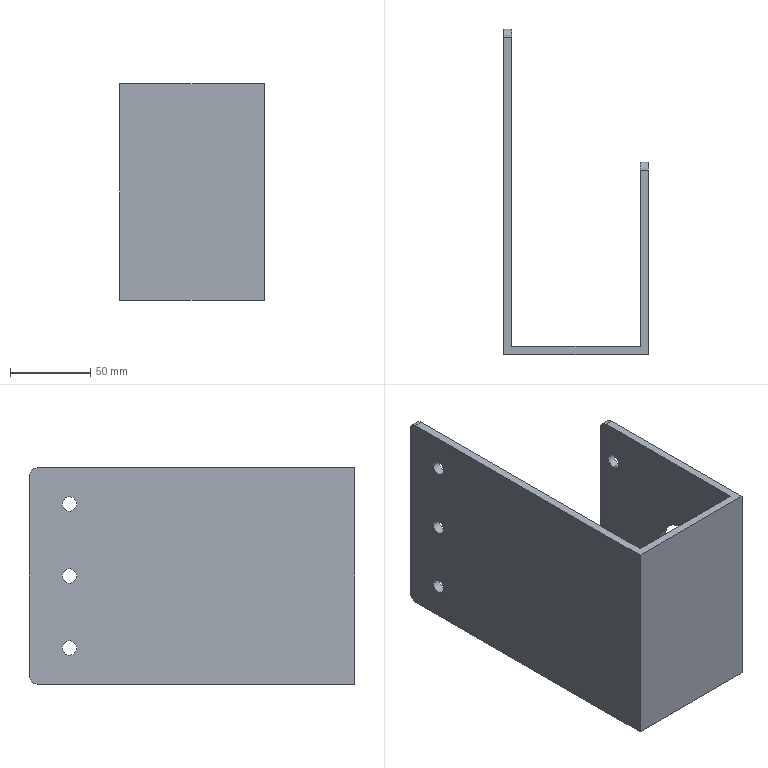Part | SolidWorks | features ICE 2, ExtruThin 1, Fillet 1 | 1 solid | 30 faces | box 90 x 203 x 135 mm | volume 261739 mm3 | cylinder 20 | plane 10 | commonest cylinder face diameters 9 x14 10 x4 45 x2
STEP:
#1=CARTESIAN_POINT('',(-35.,-32.5,-45.));
#2=VERTEX_POINT('',#1);
#3=CARTESIAN_POINT('',(-35.,-41.5,-45.));
#4=VERTEX_POINT('',#3);
#5=CARTESIAN_POINT('',(-35.,-37.,-45.));
#6=DIRECTION('',(-1.,0.,0.));
#7=DIRECTION('',(0.,1.,0.));
#8=AXIS2_PLACEMENT_3D('',#5,#6,#7);
#9=CIRCLE('',#8,4.5);
#10=EDGE_CURVE('',#2,#4,#9,.T.);
#11=ORIENTED_EDGE('',*,*,#10,.F.);
#12=CARTESIAN_POINT('',(-40.,-32.5,-45.));
#13=VERTEX_POINT('',#12);
#14=CARTESIAN_POINT('',(-30.,-32.5,-45.));
#15=DIRECTION('',(-1.,0.,0.));
#16=VECTOR('',#15,1000.);
#17=LINE('',#14,#16);
#18=EDGE_CURVE('',#2,#13,#17,.T.);
#19=ORIENTED_EDGE('',*,*,#18,.T.);
#20=CARTESIAN_POINT('',(-40.,-41.5,-45.));
#21=VERTEX_POINT('',#20);
#22=CARTESIAN_POINT('',(-40.,-37.,-45.));
#23=DIRECTION('',(1.,0.,0.));
#24=DIRECTION('',(0.,1.,0.));
#25=AXIS2_PLACEMENT_3D('',#22,#23,#24);
#26=CIRCLE('',#25,4.5);
#27=EDGE_CURVE('',#21,#13,#26,.T.);
#28=ORIENTED_EDGE('',*,*,#27,.F.);
#29=CARTESIAN_POINT('',(-30.,-41.5,-45.));
#30=DIRECTION('',(-1.,0.,0.));
#31=VECTOR('',#30,1000.);
#32=LINE('',#29,#31);
#33=EDGE_CURVE('',#4,#21,#32,.T.);
#34=ORIENTED_EDGE('',*,*,#33,.F.);
#35=EDGE_LOOP('',(#11,#19,#28,#34));
#36=FACE_OUTER_BOUND('',#35,.T.);
#37=CARTESIAN_POINT('',(-30.,-37.,-45.));
#38=DIRECTION('',(-1.,0.,0.));
#39=DIRECTION('',(0.,-1.,0.));
#40=AXIS2_PLACEMENT_3D('',#37,#38,#39);
#41=CYLINDRICAL_SURFACE('',#40,4.5);
#42=ADVANCED_FACE('',(#36),#41,.F.);
#43=CARTESIAN_POINT('',(-35.,-32.5,45.));
#44=VERTEX_POINT('',#43);
#45=CARTESIAN_POINT('',(-35.,-41.5,45.));
#46=VERTEX_POINT('',#45);
#47=CARTESIAN_POINT('',(-35.,-37.,45.));
#48=DIRECTION('',(-1.,0.,0.));
#49=DIRECTION('',(0.,1.,0.));
#50=AXIS2_PLACEMENT_3D('',#47,#48,#49);
#51=CIRCLE('',#50,4.5);
#52=EDGE_CURVE('',#44,#46,#51,.T.);
#53=ORIENTED_EDGE('',*,*,#52,.F.);
#54=CARTESIAN_POINT('',(-40.,-32.5,45.));
#55=VERTEX_POINT('',#54);
#56=CARTESIAN_POINT('',(-30.,-32.5,45.));
#57=DIRECTION('',(-1.,0.,0.));
#58=VECTOR('',#57,1000.);
#59=LINE('',#56,#58);
#60=EDGE_CURVE('',#44,#55,#59,.T.);
#61=ORIENTED_EDGE('',*,*,#60,.T.);
#62=CARTESIAN_POINT('',(-40.,-41.5,45.));
#63=VERTEX_POINT('',#62);
#64=CARTESIAN_POINT('',(-40.,-37.,45.));
#65=DIRECTION('',(1.,0.,0.));
#66=DIRECTION('',(0.,1.,0.));
#67=AXIS2_PLACEMENT_3D('',#64,#65,#66);
#68=CIRCLE('',#67,4.5);
#69=EDGE_CURVE('',#63,#55,#68,.T.);
#70=ORIENTED_EDGE('',*,*,#69,.F.);
#71=CARTESIAN_POINT('',(-30.,-41.5,45.));
#72=DIRECTION('',(-1.,0.,0.));
#73=VECTOR('',#72,1000.);
#74=LINE('',#71,#73);
#75=EDGE_CURVE('',#46,#63,#74,.T.);
#76=ORIENTED_EDGE('',*,*,#75,.F.);
#77=EDGE_LOOP('',(#53,#61,#70,#76));
#78=FACE_OUTER_BOUND('',#77,.T.);
#79=CARTESIAN_POINT('',(-30.,-37.,45.));
#80=DIRECTION('',(-1.,0.,0.));
#81=DIRECTION('',(0.,-1.,0.));
#82=AXIS2_PLACEMENT_3D('',#79,#80,#81);
#83=CYLINDRICAL_SURFACE('',#82,4.5);
#84=ADVANCED_FACE('',(#78),#83,.F.);
#85=CARTESIAN_POINT('',(-35.,-32.5,0.));
#86=VERTEX_POINT('',#85);
#87=CARTESIAN_POINT('',(-35.,-41.5,0.));
#88=VERTEX_POINT('',#87);
#89=CARTESIAN_POINT('',(-35.,-37.,0.));
#90=DIRECTION('',(-1.,0.,0.));
#91=DIRECTION('',(0.,1.,0.));
#92=AXIS2_PLACEMENT_3D('',#89,#90,#91);
#93=CIRCLE('',#92,4.5);
#94=EDGE_CURVE('',#86,#88,#93,.T.);
#95=ORIENTED_EDGE('',*,*,#94,.F.);
#96=CARTESIAN_POINT('',(-40.,-32.5,0.));
#97=VERTEX_POINT('',#96);
#98=CARTESIAN_POINT('',(-30.,-32.5,0.));
#99=DIRECTION('',(-1.,0.,0.));
#100=VECTOR('',#99,1000.);
#101=LINE('',#98,#100);
#102=EDGE_CURVE('',#86,#97,#101,.T.);
#103=ORIENTED_EDGE('',*,*,#102,.T.);
#104=CARTESIAN_POINT('',(-40.,-41.5,0.));
#105=VERTEX_POINT('',#104);
#106=CARTESIAN_POINT('',(-40.,-37.,0.));
#107=DIRECTION('',(1.,0.,0.));
#108=DIRECTION('',(0.,1.,0.));
#109=AXIS2_PLACEMENT_3D('',#106,#107,#108);
#110=CIRCLE('',#109,4.5);
#111=EDGE_CURVE('',#105,#97,#110,.T.);
#112=ORIENTED_EDGE('',*,*,#111,.F.);
#113=CARTESIAN_POINT('',(-30.,-41.5,0.));
#114=DIRECTION('',(-1.,0.,0.));
#115=VECTOR('',#114,1000.);
#116=LINE('',#113,#115);
#117=EDGE_CURVE('',#88,#105,#116,.T.);
#118=ORIENTED_EDGE('',*,*,#117,.F.);
#119=EDGE_LOOP('',(#95,#103,#112,#118));
#120=FACE_OUTER_BOUND('',#119,.T.);
#121=CARTESIAN_POINT('',(-30.,-37.,0.));
#122=DIRECTION('',(-1.,0.,0.));
#123=DIRECTION('',(0.,-1.,0.));
#124=AXIS2_PLACEMENT_3D('',#121,#122,#123);
#125=CYLINDRICAL_SURFACE('',#124,4.5);
#126=ADVANCED_FACE('',(#120),#125,.F.);
#127=CARTESIAN_POINT('',(45.,-106.574,37.926));
#128=VERTEX_POINT('',#127);
#129=CARTESIAN_POINT('',(45.,-106.574,46.926));
#130=VERTEX_POINT('',#129);
#131=CARTESIAN_POINT('',(45.,-106.574,42.426));
#132=DIRECTION('',(-1.,0.,0.));
#133=DIRECTION('',(0.,0.,1.));
#134=AXIS2_PLACEMENT_3D('',#131,#132,#133);
#135=CIRCLE('',#134,4.5);
#136=EDGE_CURVE('',#128,#130,#135,.T.);
#137=ORIENTED_EDGE('',*,*,#136,.T.);
#138=CARTESIAN_POINT('',(50.,-106.574,46.926));
#139=VERTEX_POINT('',#138);
#140=CARTESIAN_POINT('',(40.,-106.574,46.926));
#141=DIRECTION('',(1.,0.,0.));
#142=VECTOR('',#141,1000.);
#143=LINE('',#140,#142);
#144=EDGE_CURVE('',#130,#139,#143,.T.);
#145=ORIENTED_EDGE('',*,*,#144,.T.);
#146=CARTESIAN_POINT('',(50.,-106.574,37.926));
#147=VERTEX_POINT('',#146);
#148=CARTESIAN_POINT('',(50.,-106.574,42.426));
#149=DIRECTION('',(1.,0.,0.));
#150=DIRECTION('',(0.,0.,-1.));
#151=AXIS2_PLACEMENT_3D('',#148,#149,#150);
#152=CIRCLE('',#151,4.5);
#153=EDGE_CURVE('',#139,#147,#152,.T.);
#154=ORIENTED_EDGE('',*,*,#153,.T.);
#155=CARTESIAN_POINT('',(40.,-106.574,37.926));
#156=DIRECTION('',(1.,0.,0.));
#157=VECTOR('',#156,1000.);
#158=LINE('',#155,#157);
#159=EDGE_CURVE('',#128,#147,#158,.T.);
#160=ORIENTED_EDGE('',*,*,#159,.F.);
#161=EDGE_LOOP('',(#137,#145,#154,#160));
#162=FACE_OUTER_BOUND('',#161,.T.);
#163=CARTESIAN_POINT('',(40.,-106.574,42.426));
#164=DIRECTION('',(1.,0.,0.));
#165=DIRECTION('',(0.,0.,-1.));
#166=AXIS2_PLACEMENT_3D('',#163,#164,#165);
#167=CYLINDRICAL_SURFACE('',#166,4.5);
#168=ADVANCED_FACE('',(#162),#167,.F.);
#169=CARTESIAN_POINT('',(45.,-191.426,37.926));
#170=VERTEX_POINT('',#169);
#171=CARTESIAN_POINT('',(45.,-191.426,46.926));
#172=VERTEX_POINT('',#171);
#173=CARTESIAN_POINT('',(45.,-191.426,42.426));
#174=DIRECTION('',(-1.,0.,0.));
#175=DIRECTION('',(0.,0.,1.));
#176=AXIS2_PLACEMENT_3D('',#173,#174,#175);
#177=CIRCLE('',#176,4.5);
#178=EDGE_CURVE('',#170,#172,#177,.T.);
#179=ORIENTED_EDGE('',*,*,#178,.T.);
#180=CARTESIAN_POINT('',(50.,-191.426,46.926));
#181=VERTEX_POINT('',#180);
#182=CARTESIAN_POINT('',(40.,-191.426,46.926));
#183=DIRECTION('',(1.,0.,0.));
#184=VECTOR('',#183,1000.);
#185=LINE('',#182,#184);
#186=EDGE_CURVE('',#172,#181,#185,.T.);
#187=ORIENTED_EDGE('',*,*,#186,.T.);
#188=CARTESIAN_POINT('',(50.,-191.426,37.926));
#189=VERTEX_POINT('',#188);
#190=CARTESIAN_POINT('',(50.,-191.426,42.426));
#191=DIRECTION('',(1.,0.,0.));
#192=DIRECTION('',(0.,0.,-1.));
#193=AXIS2_PLACEMENT_3D('',#190,#191,#192);
#194=CIRCLE('',#193,4.5);
#195=EDGE_CURVE('',#181,#189,#194,.T.);
#196=ORIENTED_EDGE('',*,*,#195,.T.);
#197=CARTESIAN_POINT('',(40.,-191.426,37.926));
#198=DIRECTION('',(1.,0.,0.));
#199=VECTOR('',#198,1000.);
#200=LINE('',#197,#199);
#201=EDGE_CURVE('',#170,#189,#200,.T.);
#202=ORIENTED_EDGE('',*,*,#201,.F.);
#203=EDGE_LOOP('',(#179,#187,#196,#202));
#204=FACE_OUTER_BOUND('',#203,.T.);
#205=CARTESIAN_POINT('',(40.,-191.426,42.426));
#206=DIRECTION('',(1.,0.,0.));
#207=DIRECTION('',(0.,0.,-1.));
#208=AXIS2_PLACEMENT_3D('',#205,#206,#207);
#209=CYLINDRICAL_SURFACE('',#208,4.5);
#210=ADVANCED_FACE('',(#204),#209,.F.);
#211=CARTESIAN_POINT('',(45.,-191.426,-46.926));
#212=VERTEX_POINT('',#211);
#213=CARTESIAN_POINT('',(45.,-191.426,-37.926));
#214=VERTEX_POINT('',#213);
#215=CARTESIAN_POINT('',(45.,-191.426,-42.426));
#216=DIRECTION('',(-1.,0.,0.));
#217=DIRECTION('',(0.,0.,1.));
#218=AXIS2_PLACEMENT_3D('',#215,#216,#217);
#219=CIRCLE('',#218,4.5);
#220=EDGE_CURVE('',#212,#214,#219,.T.);
#221=ORIENTED_EDGE('',*,*,#220,.T.);
#222=CARTESIAN_POINT('',(50.,-191.426,-37.926));
#223=VERTEX_POINT('',#222);
#224=CARTESIAN_POINT('',(40.,-191.426,-37.926));
#225=DIRECTION('',(1.,0.,0.));
#226=VECTOR('',#225,1000.);
#227=LINE('',#224,#226);
#228=EDGE_CURVE('',#214,#223,#227,.T.);
#229=ORIENTED_EDGE('',*,*,#228,.T.);
#230=CARTESIAN_POINT('',(50.,-191.426,-46.926));
#231=VERTEX_POINT('',#230);
#232=CARTESIAN_POINT('',(50.,-191.426,-42.426));
#233=DIRECTION('',(1.,0.,0.));
#234=DIRECTION('',(0.,0.,-1.));
#235=AXIS2_PLACEMENT_3D('',#232,#233,#234);
#236=CIRCLE('',#235,4.5);
#237=EDGE_CURVE('',#223,#231,#236,.T.);
#238=ORIENTED_EDGE('',*,*,#237,.T.);
#239=CARTESIAN_POINT('',(40.,-191.426,-46.926));
#240=DIRECTION('',(1.,0.,0.));
#241=VECTOR('',#240,1000.);
#242=LINE('',#239,#241);
#243=EDGE_CURVE('',#212,#231,#242,.T.);
#244=ORIENTED_EDGE('',*,*,#243,.F.);
#245=EDGE_LOOP('',(#221,#229,#238,#244));
#246=FACE_OUTER_BOUND('',#245,.T.);
#247=CARTESIAN_POINT('',(40.,-191.426,-42.426));
#248=DIRECTION('',(1.,0.,0.));
#249=DIRECTION('',(0.,0.,-1.));
#250=AXIS2_PLACEMENT_3D('',#247,#248,#249);
#251=CYLINDRICAL_SURFACE('',#250,4.5);
#252=ADVANCED_FACE('',(#246),#251,.F.);
#253=CARTESIAN_POINT('',(45.,-106.574,-46.926));
#254=VERTEX_POINT('',#253);
#255=CARTESIAN_POINT('',(45.,-106.574,-37.926));
#256=VERTEX_POINT('',#255);
#257=CARTESIAN_POINT('',(45.,-106.574,-42.426));
#258=DIRECTION('',(-1.,0.,0.));
#259=DIRECTION('',(0.,0.,1.));
#260=AXIS2_PLACEMENT_3D('',#257,#258,#259);
#261=CIRCLE('',#260,4.5);
#262=EDGE_CURVE('',#254,#256,#261,.T.);
#263=ORIENTED_EDGE('',*,*,#262,.T.);
#264=CARTESIAN_POINT('',(50.,-106.574,-37.926));
#265=VERTEX_POINT('',#264);
#266=CARTESIAN_POINT('',(40.,-106.574,-37.926));
#267=DIRECTION('',(1.,0.,0.));
#268=VECTOR('',#267,1000.);
#269=LINE('',#266,#268);
#270=EDGE_CURVE('',#256,#265,#269,.T.);
#271=ORIENTED_EDGE('',*,*,#270,.T.);
#272=CARTESIAN_POINT('',(50.,-106.574,-46.926));
#273=VERTEX_POINT('',#272);
#274=CARTESIAN_POINT('',(50.,-106.574,-42.426));
#275=DIRECTION('',(1.,0.,0.));
#276=DIRECTION('',(0.,0.,-1.));
#277=AXIS2_PLACEMENT_3D('',#274,#275,#276);
#278=CIRCLE('',#277,4.5);
#279=EDGE_CURVE('',#265,#273,#278,.T.);
#280=ORIENTED_EDGE('',*,*,#279,.T.);
#281=CARTESIAN_POINT('',(40.,-106.574,-46.926));
#282=DIRECTION('',(1.,0.,0.));
#283=VECTOR('',#282,1000.);
#284=LINE('',#281,#283);
#285=EDGE_CURVE('',#254,#273,#284,.T.);
#286=ORIENTED_EDGE('',*,*,#285,.F.);
#287=EDGE_LOOP('',(#263,#271,#280,#286));
#288=FACE_OUTER_BOUND('',#287,.T.);
#289=CARTESIAN_POINT('',(40.,-106.574,-42.426));
#290=DIRECTION('',(1.,0.,0.));
#291=DIRECTION('',(0.,0.,-1.));
#292=AXIS2_PLACEMENT_3D('',#289,#290,#291);
#293=CYLINDRICAL_SURFACE('',#292,4.5);
#294=ADVANCED_FACE('',(#288),#293,.F.);
#295=CARTESIAN_POINT('',(45.,-169.,-22.5));
#296=VERTEX_POINT('',#295);
#297=CARTESIAN_POINT('',(45.,-169.,22.5));
#298=VERTEX_POINT('',#297);
#299=CARTESIAN_POINT('',(45.,-169.,0.));
#300=DIRECTION('',(-1.,0.,0.));
#301=DIRECTION('',(0.,0.,1.));
#302=AXIS2_PLACEMENT_3D('',#299,#300,#301);
#303=CIRCLE('',#302,22.5);
#304=EDGE_CURVE('',#296,#298,#303,.T.);
#305=ORIENTED_EDGE('',*,*,#304,.T.);
#306=CARTESIAN_POINT('',(50.,-169.,22.5));
#307=VERTEX_POINT('',#306);
#308=CARTESIAN_POINT('',(40.,-169.,22.5));
#309=DIRECTION('',(1.,0.,0.));
#310=VECTOR('',#309,1000.);
#311=LINE('',#308,#310);
#312=EDGE_CURVE('',#298,#307,#311,.T.);
#313=ORIENTED_EDGE('',*,*,#312,.T.);
#314=CARTESIAN_POINT('',(50.,-169.,-22.5));
#315=VERTEX_POINT('',#314);
#316=CARTESIAN_POINT('',(50.,-169.,0.));
#317=DIRECTION('',(1.,0.,0.));
#318=DIRECTION('',(0.,0.,-1.));
#319=AXIS2_PLACEMENT_3D('',#316,#317,#318);
#320=CIRCLE('',#319,22.5);
#321=EDGE_CURVE('',#307,#315,#320,.T.);
#322=ORIENTED_EDGE('',*,*,#321,.T.);
#323=CARTESIAN_POINT('',(40.,-169.,-22.5));
#324=DIRECTION('',(1.,0.,0.));
#325=VECTOR('',#324,1000.);
#326=LINE('',#323,#325);
#327=EDGE_CURVE('',#296,#315,#326,.T.);
#328=ORIENTED_EDGE('',*,*,#327,.F.);
#329=EDGE_LOOP('',(#305,#313,#322,#328));
#330=FACE_OUTER_BOUND('',#329,.T.);
#331=CARTESIAN_POINT('',(40.,-169.,0.));
#332=DIRECTION('',(1.,0.,0.));
#333=DIRECTION('',(0.,0.,-1.));
#334=AXIS2_PLACEMENT_3D('',#331,#332,#333);
#335=CYLINDRICAL_SURFACE('',#334,22.5);
#336=ADVANCED_FACE('',(#330),#335,.F.);
#337=CARTESIAN_POINT('',(50.,-106.574,42.426));
#338=DIRECTION('',(1.,0.,0.));
#339=DIRECTION('',(0.,0.,-1.));
#340=AXIS2_PLACEMENT_3D('',#337,#338,#339);
#341=CIRCLE('',#340,4.5);
#342=EDGE_CURVE('',#147,#139,#341,.T.);
#343=ORIENTED_EDGE('',*,*,#342,.F.);
#344=ORIENTED_EDGE('',*,*,#153,.F.);
#345=EDGE_LOOP('',(#343,#344));
#346=FACE_BOUND('',#345,.T.);
#347=CARTESIAN_POINT('',(50.,-191.426,42.426));
#348=DIRECTION('',(1.,0.,0.));
#349=DIRECTION('',(0.,0.,-1.));
#350=AXIS2_PLACEMENT_3D('',#347,#348,#349);
#351=CIRCLE('',#350,4.5);
#352=EDGE_CURVE('',#189,#181,#351,.T.);
#353=ORIENTED_EDGE('',*,*,#352,.F.);
#354=ORIENTED_EDGE('',*,*,#195,.F.);
#355=EDGE_LOOP('',(#353,#354));
#356=FACE_BOUND('',#355,.T.);
#357=CARTESIAN_POINT('',(50.,-191.426,-42.426));
#358=DIRECTION('',(1.,0.,0.));
#359=DIRECTION('',(0.,0.,-1.));
#360=AXIS2_PLACEMENT_3D('',#357,#358,#359);
#361=CIRCLE('',#360,4.5);
#362=EDGE_CURVE('',#231,#223,#361,.T.);
#363=ORIENTED_EDGE('',*,*,#362,.F.);
#364=ORIENTED_EDGE('',*,*,#237,.F.);
#365=EDGE_LOOP('',(#363,#364));
#366=FACE_BOUND('',#365,.T.);
#367=CARTESIAN_POINT('',(50.,-106.574,-42.426));
#368=DIRECTION('',(1.,0.,0.));
#369=DIRECTION('',(0.,0.,-1.));
#370=AXIS2_PLACEMENT_3D('',#367,#368,#369);
#371=CIRCLE('',#370,4.5);
#372=EDGE_CURVE('',#273,#265,#371,.T.);
#373=ORIENTED_EDGE('',*,*,#372,.F.);
#374=ORIENTED_EDGE('',*,*,#279,.F.);
#375=EDGE_LOOP('',(#373,#374));
#376=FACE_BOUND('',#375,.T.);
#377=CARTESIAN_POINT('',(50.,-169.,0.));
#378=DIRECTION('',(1.,0.,0.));
#379=DIRECTION('',(0.,0.,-1.));
#380=AXIS2_PLACEMENT_3D('',#377,#378,#379);
#381=CIRCLE('',#380,22.5);
#382=EDGE_CURVE('',#315,#307,#381,.T.);
#383=ORIENTED_EDGE('',*,*,#382,.F.);
#384=ORIENTED_EDGE('',*,*,#321,.F.);
#385=EDGE_LOOP('',(#383,#384));
#386=FACE_BOUND('',#385,.T.);
#387=CARTESIAN_POINT('',(50.,-215.,-67.5));
#388=VERTEX_POINT('',#387);
#389=CARTESIAN_POINT('',(50.,-100.,-67.5));
#390=VERTEX_POINT('',#389);
#391=CARTESIAN_POINT('',(50.,-215.,-67.5));
#392=DIRECTION('',(0.,1.,0.));
#393=VECTOR('',#392,1000.);
#394=LINE('',#391,#393);
#395=EDGE_CURVE('',#388,#390,#394,.T.);
#396=ORIENTED_EDGE('',*,*,#395,.T.);
#397=CARTESIAN_POINT('',(50.,-95.,-62.5));
#398=VERTEX_POINT('',#397);
#399=CARTESIAN_POINT('',(50.,-100.,-62.5));
#400=DIRECTION('',(1.,0.,0.));
#401=DIRECTION('',(0.,0.,1.));
#402=AXIS2_PLACEMENT_3D('',#399,#400,#401);
#403=CIRCLE('',#402,5.);
#404=EDGE_CURVE('',#390,#398,#403,.T.);
#405=ORIENTED_EDGE('',*,*,#404,.T.);
#406=CARTESIAN_POINT('',(50.,-95.,62.5));
#407=VERTEX_POINT('',#406);
#408=CARTESIAN_POINT('',(50.,-95.,67.5));
#409=DIRECTION('',(0.,0.,-1.));
#410=VECTOR('',#409,1000.);
#411=LINE('',#408,#410);
#412=EDGE_CURVE('',#407,#398,#411,.T.);
#413=ORIENTED_EDGE('',*,*,#412,.F.);
#414=CARTESIAN_POINT('',(50.,-100.,67.5));
#415=VERTEX_POINT('',#414);
#416=CARTESIAN_POINT('',(50.,-100.,62.5));
#417=DIRECTION('',(1.,0.,0.));
#418=DIRECTION('',(0.,0.,1.));
#419=AXIS2_PLACEMENT_3D('',#416,#417,#418);
#420=CIRCLE('',#419,5.);
#421=EDGE_CURVE('',#407,#415,#420,.T.);
#422=ORIENTED_EDGE('',*,*,#421,.T.);
#423=CARTESIAN_POINT('',(50.,-215.,67.5));
#424=VERTEX_POINT('',#423);
#425=CARTESIAN_POINT('',(50.,-215.,67.5));
#426=DIRECTION('',(0.,1.,0.));
#427=VECTOR('',#426,1000.);
#428=LINE('',#425,#427);
#429=EDGE_CURVE('',#424,#415,#428,.T.);
#430=ORIENTED_EDGE('',*,*,#429,.F.);
#431=CARTESIAN_POINT('',(50.,-215.,67.5));
#432=DIRECTION('',(0.,0.,-1.));
#433=VECTOR('',#432,1000.);
#434=LINE('',#431,#433);
#435=EDGE_CURVE('',#424,#388,#434,.T.);
#436=ORIENTED_EDGE('',*,*,#435,.T.);
#437=EDGE_LOOP('',(#396,#405,#413,#422,#430,#436));
#438=FACE_OUTER_BOUND('',#437,.T.);
#439=CARTESIAN_POINT('',(50.,-215.,67.5));
#440=DIRECTION('',(-1.,0.,0.));
#441=DIRECTION('',(0.,0.,1.));
#442=AXIS2_PLACEMENT_3D('',#439,#440,#441);
#443=PLANE('',#442);
#444=ADVANCED_FACE('',(#346,#356,#366,#376,#386,#438),#443,.F.);
#445=ORIENTED_EDGE('',*,*,#412,.T.);
#446=CARTESIAN_POINT('',(45.,-95.,-62.5));
#447=VERTEX_POINT('',#446);
#448=CARTESIAN_POINT('',(45.,-95.,-62.5));
#449=DIRECTION('',(-1.,0.,0.));
#450=VECTOR('',#449,1000.);
#451=LINE('',#448,#450);
#452=EDGE_CURVE('',#398,#447,#451,.T.);
#453=ORIENTED_EDGE('',*,*,#452,.T.);
#454=CARTESIAN_POINT('',(45.,-95.,62.5));
#455=VERTEX_POINT('',#454);
#456=CARTESIAN_POINT('',(45.,-95.,67.5));
#457=DIRECTION('',(0.,0.,-1.));
#458=VECTOR('',#457,1000.);
#459=LINE('',#456,#458);
#460=EDGE_CURVE('',#455,#447,#459,.T.);
#461=ORIENTED_EDGE('',*,*,#460,.F.);
#462=CARTESIAN_POINT('',(50.,-95.,62.5));
#463=DIRECTION('',(1.,0.,0.));
#464=VECTOR('',#463,1000.);
#465=LINE('',#462,#464);
#466=EDGE_CURVE('',#455,#407,#465,.T.);
#467=ORIENTED_EDGE('',*,*,#466,.T.);
#468=EDGE_LOOP('',(#445,#453,#461,#467));
#469=FACE_OUTER_BOUND('',#468,.T.);
#470=CARTESIAN_POINT('',(45.,-95.,67.5));
#471=DIRECTION('',(0.,1.,0.));
#472=DIRECTION('',(0.,0.,1.));
#473=AXIS2_PLACEMENT_3D('',#470,#471,#472);
#474=PLANE('',#473);
#475=ADVANCED_FACE('',(#469),#474,.T.);
#476=ORIENTED_EDGE('',*,*,#136,.F.);
#477=CARTESIAN_POINT('',(45.,-106.574,42.426));
#478=DIRECTION('',(-1.,0.,0.));
#479=DIRECTION('',(0.,0.,1.));
#480=AXIS2_PLACEMENT_3D('',#477,#478,#479);
#481=CIRCLE('',#480,4.5);
#482=EDGE_CURVE('',#130,#128,#481,.T.);
#483=ORIENTED_EDGE('',*,*,#482,.F.);
#484=EDGE_LOOP('',(#476,#483));
#485=FACE_BOUND('',#484,.T.);
#486=ORIENTED_EDGE('',*,*,#178,.F.);
#487=CARTESIAN_POINT('',(45.,-191.426,42.426));
#488=DIRECTION('',(-1.,0.,0.));
#489=DIRECTION('',(0.,0.,1.));
#490=AXIS2_PLACEMENT_3D('',#487,#488,#489);
#491=CIRCLE('',#490,4.5);
#492=EDGE_CURVE('',#172,#170,#491,.T.);
#493=ORIENTED_EDGE('',*,*,#492,.F.);
#494=EDGE_LOOP('',(#486,#493));
#495=FACE_BOUND('',#494,.T.);
#496=ORIENTED_EDGE('',*,*,#220,.F.);
#497=CARTESIAN_POINT('',(45.,-191.426,-42.426));
#498=DIRECTION('',(-1.,0.,0.));
#499=DIRECTION('',(0.,0.,1.));
#500=AXIS2_PLACEMENT_3D('',#497,#498,#499);
#501=CIRCLE('',#500,4.5);
#502=EDGE_CURVE('',#214,#212,#501,.T.);
#503=ORIENTED_EDGE('',*,*,#502,.F.);
#504=EDGE_LOOP('',(#496,#503));
#505=FACE_BOUND('',#504,.T.);
#506=ORIENTED_EDGE('',*,*,#262,.F.);
#507=CARTESIAN_POINT('',(45.,-106.574,-42.426));
#508=DIRECTION('',(-1.,0.,0.));
#509=DIRECTION('',(0.,0.,1.));
#510=AXIS2_PLACEMENT_3D('',#507,#508,#509);
#511=CIRCLE('',#510,4.5);
#512=EDGE_CURVE('',#256,#254,#511,.T.);
#513=ORIENTED_EDGE('',*,*,#512,.F.);
#514=EDGE_LOOP('',(#506,#513));
#515=FACE_BOUND('',#514,.T.);
#516=ORIENTED_EDGE('',*,*,#304,.F.);
#517=CARTESIAN_POINT('',(45.,-169.,0.));
#518=DIRECTION('',(-1.,0.,0.));
#519=DIRECTION('',(0.,0.,1.));
#520=AXIS2_PLACEMENT_3D('',#517,#518,#519);
#521=CIRCLE('',#520,22.5);
#522=EDGE_CURVE('',#298,#296,#521,.T.);
#523=ORIENTED_EDGE('',*,*,#522,.F.);
#524=EDGE_LOOP('',(#516,#523));
#525=FACE_BOUND('',#524,.T.);
#526=ORIENTED_EDGE('',*,*,#460,.T.);
#527=CARTESIAN_POINT('',(45.,-100.,-67.5));
#528=VERTEX_POINT('',#527);
#529=CARTESIAN_POINT('',(45.,-100.,-62.5));
#530=DIRECTION('',(-1.,0.,0.));
#531=DIRECTION('',(0.,0.,1.));
#532=AXIS2_PLACEMENT_3D('',#529,#530,#531);
#533=CIRCLE('',#532,5.);
#534=EDGE_CURVE('',#447,#528,#533,.T.);
#535=ORIENTED_EDGE('',*,*,#534,.T.);
#536=CARTESIAN_POINT('',(45.,-210.,-67.5));
#537=VERTEX_POINT('',#536);
#538=CARTESIAN_POINT('',(45.,-215.,-67.5));
#539=DIRECTION('',(0.,1.,0.));
#540=VECTOR('',#539,1000.);
#541=LINE('',#538,#540);
#542=EDGE_CURVE('',#537,#528,#541,.T.);
#543=ORIENTED_EDGE('',*,*,#542,.F.);
#544=CARTESIAN_POINT('',(45.,-210.,67.5));
#545=VERTEX_POINT('',#544);
#546=CARTESIAN_POINT('',(45.,-210.,67.5));
#547=DIRECTION('',(0.,0.,-1.));
#548=VECTOR('',#547,1000.);
#549=LINE('',#546,#548);
#550=EDGE_CURVE('',#545,#537,#549,.T.);
#551=ORIENTED_EDGE('',*,*,#550,.F.);
#552=CARTESIAN_POINT('',(45.,-100.,67.5));
#553=VERTEX_POINT('',#552);
#554=CARTESIAN_POINT('',(45.,-215.,67.5));
#555=DIRECTION('',(0.,1.,0.));
#556=VECTOR('',#555,1000.);
#557=LINE('',#554,#556);
#558=EDGE_CURVE('',#545,#553,#557,.T.);
#559=ORIENTED_EDGE('',*,*,#558,.T.);
#560=CARTESIAN_POINT('',(45.,-100.,62.5));
#561=DIRECTION('',(-1.,0.,0.));
#562=DIRECTION('',(0.,0.,1.));
#563=AXIS2_PLACEMENT_3D('',#560,#561,#562);
#564=CIRCLE('',#563,5.);
#565=EDGE_CURVE('',#553,#455,#564,.T.);
#566=ORIENTED_EDGE('',*,*,#565,.T.);
#567=EDGE_LOOP('',(#526,#535,#543,#551,#559,#566));
#568=FACE_OUTER_BOUND('',#567,.T.);
#569=CARTESIAN_POINT('',(45.,-215.,67.5));
#570=DIRECTION('',(-1.,0.,0.));
#571=DIRECTION('',(0.,0.,1.));
#572=AXIS2_PLACEMENT_3D('',#569,#570,#571);
#573=PLANE('',#572);
#574=ADVANCED_FACE('',(#485,#495,#505,#515,#525,#568),#573,.T.);
#575=CARTESIAN_POINT('',(-35.,-210.,-67.5));
#576=VERTEX_POINT('',#575);
#577=CARTESIAN_POINT('',(-40.,-210.,-67.5));
#578=DIRECTION('',(1.,0.,0.));
#579=VECTOR('',#578,1000.);
#580=LINE('',#577,#579);
#581=EDGE_CURVE('',#576,#537,#580,.T.);
#582=ORIENTED_EDGE('',*,*,#581,.F.);
#583=CARTESIAN_POINT('',(-35.,-210.,67.5));
#584=VERTEX_POINT('',#583);
#585=CARTESIAN_POINT('',(-35.,-210.,67.5));
#586=DIRECTION('',(0.,0.,-1.));
#587=VECTOR('',#586,1000.);
#588=LINE('',#585,#587);
#589=EDGE_CURVE('',#584,#576,#588,.T.);
#590=ORIENTED_EDGE('',*,*,#589,.F.);
#591=CARTESIAN_POINT('',(-40.,-210.,67.5));
#592=DIRECTION('',(1.,0.,0.));
#593=VECTOR('',#592,1000.);
#594=LINE('',#591,#593);
#595=EDGE_CURVE('',#584,#545,#594,.T.);
#596=ORIENTED_EDGE('',*,*,#595,.T.);
#597=ORIENTED_EDGE('',*,*,#550,.T.);
#598=EDGE_LOOP('',(#582,#590,#596,#597));
#599=FACE_OUTER_BOUND('',#598,.T.);
#600=CARTESIAN_POINT('',(-40.,-210.,67.5));
#601=DIRECTION('',(0.,1.,0.));
#602=DIRECTION('',(0.,0.,1.));
#603=AXIS2_PLACEMENT_3D('',#600,#601,#602);
#604=PLANE('',#603);
#605=ADVANCED_FACE('',(#599),#604,.T.);
#606=CARTESIAN_POINT('',(-35.,-37.,-45.));
#607=DIRECTION('',(-1.,0.,0.));
#608=DIRECTION('',(0.,1.,0.));
#609=AXIS2_PLACEMENT_3D('',#606,#607,#608);
#610=CIRCLE('',#609,4.5);
#611=EDGE_CURVE('',#4,#2,#610,.T.);
#612=ORIENTED_EDGE('',*,*,#611,.T.);
#613=ORIENTED_EDGE('',*,*,#10,.T.);
#614=EDGE_LOOP('',(#612,#613));
#615=FACE_BOUND('',#614,.T.);
#616=CARTESIAN_POINT('',(-35.,-37.,45.));
#617=DIRECTION('',(-1.,0.,0.));
#618=DIRECTION('',(0.,1.,0.));
#619=AXIS2_PLACEMENT_3D('',#616,#617,#618);
#620=CIRCLE('',#619,4.5);
#621=EDGE_CURVE('',#46,#44,#620,.T.);
#622=ORIENTED_EDGE('',*,*,#621,.T.);
#623=ORIENTED_EDGE('',*,*,#52,.T.);
#624=EDGE_LOOP('',(#622,#623));
#625=FACE_BOUND('',#624,.T.);
#626=CARTESIAN_POINT('',(-35.,-37.,0.));
#627=DIRECTION('',(-1.,0.,0.));
#628=DIRECTION('',(0.,1.,0.));
#629=AXIS2_PLACEMENT_3D('',#626,#627,#628);
#630=CIRCLE('',#629,4.5);
#631=EDGE_CURVE('',#88,#86,#630,.T.);
#632=ORIENTED_EDGE('',*,*,#631,.T.);
#633=ORIENTED_EDGE('',*,*,#94,.T.);
#634=EDGE_LOOP('',(#632,#633));
#635=FACE_BOUND('',#634,.T.);
#636=CARTESIAN_POINT('',(-35.,-17.,-67.5));
#637=VERTEX_POINT('',#636);
#638=CARTESIAN_POINT('',(-35.,-12.,-67.5));
#639=DIRECTION('',(0.,-1.,0.));
#640=VECTOR('',#639,1000.);
#641=LINE('',#638,#640);
#642=EDGE_CURVE('',#637,#576,#641,.T.);
#643=ORIENTED_EDGE('',*,*,#642,.F.);
#644=CARTESIAN_POINT('',(-35.,-12.,-62.5));
#645=VERTEX_POINT('',#644);
#646=CARTESIAN_POINT('',(-35.,-17.,-62.5));
#647=DIRECTION('',(1.,0.,0.));
#648=DIRECTION('',(0.,1.,0.));
#649=AXIS2_PLACEMENT_3D('',#646,#647,#648);
#650=CIRCLE('',#649,5.);
#651=EDGE_CURVE('',#637,#645,#650,.T.);
#652=ORIENTED_EDGE('',*,*,#651,.T.);
#653=CARTESIAN_POINT('',(-35.,-12.,62.5));
#654=VERTEX_POINT('',#653);
#655=CARTESIAN_POINT('',(-35.,-12.,67.5));
#656=DIRECTION('',(0.,0.,-1.));
#657=VECTOR('',#656,1000.);
#658=LINE('',#655,#657);
#659=EDGE_CURVE('',#654,#645,#658,.T.);
#660=ORIENTED_EDGE('',*,*,#659,.F.);
#661=CARTESIAN_POINT('',(-35.,-17.,67.5));
#662=VERTEX_POINT('',#661);
#663=CARTESIAN_POINT('',(-35.,-17.,62.5));
#664=DIRECTION('',(1.,0.,0.));
#665=DIRECTION('',(0.,1.,0.));
#666=AXIS2_PLACEMENT_3D('',#663,#664,#665);
#667=CIRCLE('',#666,5.);
#668=EDGE_CURVE('',#654,#662,#667,.T.);
#669=ORIENTED_EDGE('',*,*,#668,.T.);
#670=CARTESIAN_POINT('',(-35.,-12.,67.5));
#671=DIRECTION('',(0.,-1.,0.));
#672=VECTOR('',#671,1000.);
#673=LINE('',#670,#672);
#674=EDGE_CURVE('',#662,#584,#673,.T.);
#675=ORIENTED_EDGE('',*,*,#674,.T.);
#676=ORIENTED_EDGE('',*,*,#589,.T.);
#677=EDGE_LOOP('',(#643,#652,#660,#669,#675,#676));
#678=FACE_OUTER_BOUND('',#677,.T.);
#679=CARTESIAN_POINT('',(-35.,-12.,67.5));
#680=DIRECTION('',(1.,0.,0.));
#681=DIRECTION('',(0.,1.,0.));
#682=AXIS2_PLACEMENT_3D('',#679,#680,#681);
#683=PLANE('',#682);
#684=ADVANCED_FACE('',(#615,#625,#635,#678),#683,.T.);
#685=ORIENTED_EDGE('',*,*,#659,.T.);
#686=CARTESIAN_POINT('',(-40.,-12.,-62.5));
#687=VERTEX_POINT('',#686);
#688=CARTESIAN_POINT('',(-40.,-12.,-62.5));
#689=DIRECTION('',(-1.,0.,0.));
#690=VECTOR('',#689,1000.);
#691=LINE('',#688,#690);
#692=EDGE_CURVE('',#645,#687,#691,.T.);
#693=ORIENTED_EDGE('',*,*,#692,.T.);
#694=CARTESIAN_POINT('',(-40.,-12.,62.5));
#695=VERTEX_POINT('',#694);
#696=CARTESIAN_POINT('',(-40.,-12.,67.5));
#697=DIRECTION('',(0.,0.,-1.));
#698=VECTOR('',#697,1000.);
#699=LINE('',#696,#698);
#700=EDGE_CURVE('',#695,#687,#699,.T.);
#701=ORIENTED_EDGE('',*,*,#700,.F.);
#702=CARTESIAN_POINT('',(-35.,-12.,62.5));
#703=DIRECTION('',(1.,0.,0.));
#704=VECTOR('',#703,1000.);
#705=LINE('',#702,#704);
#706=EDGE_CURVE('',#695,#654,#705,.T.);
#707=ORIENTED_EDGE('',*,*,#706,.T.);
#708=EDGE_LOOP('',(#685,#693,#701,#707));
#709=FACE_OUTER_BOUND('',#708,.T.);
#710=CARTESIAN_POINT('',(-40.,-12.,67.5));
#711=DIRECTION('',(0.,1.,0.));
#712=DIRECTION('',(0.,0.,1.));
#713=AXIS2_PLACEMENT_3D('',#710,#711,#712);
#714=PLANE('',#713);
#715=ADVANCED_FACE('',(#709),#714,.T.);
#716=ORIENTED_EDGE('',*,*,#27,.T.);
#717=CARTESIAN_POINT('',(-40.,-37.,-45.));
#718=DIRECTION('',(1.,0.,0.));
#719=DIRECTION('',(0.,1.,0.));
#720=AXIS2_PLACEMENT_3D('',#717,#718,#719);
#721=CIRCLE('',#720,4.5);
#722=EDGE_CURVE('',#13,#21,#721,.T.);
#723=ORIENTED_EDGE('',*,*,#722,.T.);
#724=EDGE_LOOP('',(#716,#723));
#725=FACE_BOUND('',#724,.T.);
#726=ORIENTED_EDGE('',*,*,#69,.T.);
#727=CARTESIAN_POINT('',(-40.,-37.,45.));
#728=DIRECTION('',(1.,0.,0.));
#729=DIRECTION('',(0.,1.,0.));
#730=AXIS2_PLACEMENT_3D('',#727,#728,#729);
#731=CIRCLE('',#730,4.5);
#732=EDGE_CURVE('',#55,#63,#731,.T.);
#733=ORIENTED_EDGE('',*,*,#732,.T.);
#734=EDGE_LOOP('',(#726,#733));
#735=FACE_BOUND('',#734,.T.);
#736=ORIENTED_EDGE('',*,*,#111,.T.);
#737=CARTESIAN_POINT('',(-40.,-37.,0.));
#738=DIRECTION('',(1.,0.,0.));
#739=DIRECTION('',(0.,1.,0.));
#740=AXIS2_PLACEMENT_3D('',#737,#738,#739);
#741=CIRCLE('',#740,4.5);
#742=EDGE_CURVE('',#97,#105,#741,.T.);
#743=ORIENTED_EDGE('',*,*,#742,.T.);
#744=EDGE_LOOP('',(#736,#743));
#745=FACE_BOUND('',#744,.T.);
#746=ORIENTED_EDGE('',*,*,#700,.T.);
#747=CARTESIAN_POINT('',(-40.,-17.,-67.5));
#748=VERTEX_POINT('',#747);
#749=CARTESIAN_POINT('',(-40.,-17.,-62.5));
#750=DIRECTION('',(-1.,0.,0.));
#751=DIRECTION('',(0.,1.,0.));
#752=AXIS2_PLACEMENT_3D('',#749,#750,#751);
#753=CIRCLE('',#752,5.);
#754=EDGE_CURVE('',#687,#748,#753,.T.);
#755=ORIENTED_EDGE('',*,*,#754,.T.);
#756=CARTESIAN_POINT('',(-40.,-215.,-67.5));
#757=VERTEX_POINT('',#756);
#758=CARTESIAN_POINT('',(-40.,-12.,-67.5));
#759=DIRECTION('',(0.,-1.,0.));
#760=VECTOR('',#759,1000.);
#761=LINE('',#758,#760);
#762=EDGE_CURVE('',#748,#757,#761,.T.);
#763=ORIENTED_EDGE('',*,*,#762,.T.);
#764=CARTESIAN_POINT('',(-40.,-215.,67.5));
#765=VERTEX_POINT('',#764);
#766=CARTESIAN_POINT('',(-40.,-215.,67.5));
#767=DIRECTION('',(0.,0.,-1.));
#768=VECTOR('',#767,1000.);
#769=LINE('',#766,#768);
#770=EDGE_CURVE('',#765,#757,#769,.T.);
#771=ORIENTED_EDGE('',*,*,#770,.F.);
#772=CARTESIAN_POINT('',(-40.,-17.,67.5));
#773=VERTEX_POINT('',#772);
#774=CARTESIAN_POINT('',(-40.,-12.,67.5));
#775=DIRECTION('',(0.,-1.,0.));
#776=VECTOR('',#775,1000.);
#777=LINE('',#774,#776);
#778=EDGE_CURVE('',#773,#765,#777,.T.);
#779=ORIENTED_EDGE('',*,*,#778,.F.);
#780=CARTESIAN_POINT('',(-40.,-17.,62.5));
#781=DIRECTION('',(-1.,0.,0.));
#782=DIRECTION('',(0.,1.,0.));
#783=AXIS2_PLACEMENT_3D('',#780,#781,#782);
#784=CIRCLE('',#783,5.);
#785=EDGE_CURVE('',#773,#695,#784,.T.);
#786=ORIENTED_EDGE('',*,*,#785,.T.);
#787=EDGE_LOOP('',(#746,#755,#763,#771,#779,#786));
#788=FACE_OUTER_BOUND('',#787,.T.);
#789=CARTESIAN_POINT('',(-40.,-12.,67.5));
#790=DIRECTION('',(1.,0.,0.));
#791=DIRECTION('',(0.,1.,0.));
#792=AXIS2_PLACEMENT_3D('',#789,#790,#791);
#793=PLANE('',#792);
#794=ADVANCED_FACE('',(#725,#735,#745,#788),#793,.F.);
#795=CARTESIAN_POINT('',(-40.,-215.,-67.5));
#796=DIRECTION('',(1.,0.,0.));
#797=VECTOR('',#796,1000.);
#798=LINE('',#795,#797);
#799=EDGE_CURVE('',#757,#388,#798,.T.);
#800=ORIENTED_EDGE('',*,*,#799,.T.);
#801=ORIENTED_EDGE('',*,*,#435,.F.);
#802=CARTESIAN_POINT('',(-40.,-215.,67.5));
#803=DIRECTION('',(1.,0.,0.));
#804=VECTOR('',#803,1000.);
#805=LINE('',#802,#804);
#806=EDGE_CURVE('',#765,#424,#805,.T.);
#807=ORIENTED_EDGE('',*,*,#806,.F.);
#808=ORIENTED_EDGE('',*,*,#770,.T.);
#809=EDGE_LOOP('',(#800,#801,#807,#808));
#810=FACE_OUTER_BOUND('',#809,.T.);
#811=CARTESIAN_POINT('',(-40.,-215.,67.5));
#812=DIRECTION('',(0.,1.,0.));
#813=DIRECTION('',(0.,0.,1.));
#814=AXIS2_PLACEMENT_3D('',#811,#812,#813);
#815=PLANE('',#814);
#816=ADVANCED_FACE('',(#810),#815,.F.);
#817=ORIENTED_EDGE('',*,*,#429,.T.);
#818=CARTESIAN_POINT('',(45.,-100.,67.5));
#819=DIRECTION('',(-1.,0.,0.));
#820=VECTOR('',#819,1000.);
#821=LINE('',#818,#820);
#822=EDGE_CURVE('',#415,#553,#821,.T.);
#823=ORIENTED_EDGE('',*,*,#822,.T.);
#824=ORIENTED_EDGE('',*,*,#558,.F.);
#825=ORIENTED_EDGE('',*,*,#595,.F.);
#826=ORIENTED_EDGE('',*,*,#674,.F.);
#827=CARTESIAN_POINT('',(-40.,-17.,67.5));
#828=DIRECTION('',(-1.,0.,0.));
#829=VECTOR('',#828,1000.);
#830=LINE('',#827,#829);
#831=EDGE_CURVE('',#662,#773,#830,.T.);
#832=ORIENTED_EDGE('',*,*,#831,.T.);
#833=ORIENTED_EDGE('',*,*,#778,.T.);
#834=ORIENTED_EDGE('',*,*,#806,.T.);
#835=EDGE_LOOP('',(#817,#823,#824,#825,#826,#832,#833,#834));
#836=FACE_OUTER_BOUND('',#835,.T.);
#837=CARTESIAN_POINT('',(0.,0.,67.5));
#838=DIRECTION('',(0.,0.,-1.));
#839=DIRECTION('',(-1.,0.,0.));
#840=AXIS2_PLACEMENT_3D('',#837,#838,#839);
#841=PLANE('',#840);
#842=ADVANCED_FACE('',(#836),#841,.F.);
#843=ORIENTED_EDGE('',*,*,#542,.T.);
#844=CARTESIAN_POINT('',(0.,-100.,-67.5));
#845=DIRECTION('',(1.,0.,0.));
#846=VECTOR('',#845,1000.);
#847=LINE('',#844,#846);
#848=EDGE_CURVE('',#528,#390,#847,.T.);
#849=ORIENTED_EDGE('',*,*,#848,.T.);
#850=ORIENTED_EDGE('',*,*,#395,.F.);
#851=ORIENTED_EDGE('',*,*,#799,.F.);
#852=ORIENTED_EDGE('',*,*,#762,.F.);
#853=CARTESIAN_POINT('',(0.,-17.,-67.5));
#854=DIRECTION('',(1.,0.,0.));
#855=VECTOR('',#854,1000.);
#856=LINE('',#853,#855);
#857=EDGE_CURVE('',#748,#637,#856,.T.);
#858=ORIENTED_EDGE('',*,*,#857,.T.);
#859=ORIENTED_EDGE('',*,*,#642,.T.);
#860=ORIENTED_EDGE('',*,*,#581,.T.);
#861=EDGE_LOOP('',(#843,#849,#850,#851,#852,#858,#859,#860));
#862=FACE_OUTER_BOUND('',#861,.T.);
#863=CARTESIAN_POINT('',(0.,0.,-67.5));
#864=DIRECTION('',(0.,0.,-1.));
#865=DIRECTION('',(-1.,0.,0.));
#866=AXIS2_PLACEMENT_3D('',#863,#864,#865);
#867=PLANE('',#866);
#868=ADVANCED_FACE('',(#862),#867,.T.);
#869=ORIENTED_EDGE('',*,*,#312,.F.);
#870=ORIENTED_EDGE('',*,*,#522,.T.);
#871=ORIENTED_EDGE('',*,*,#327,.T.);
#872=ORIENTED_EDGE('',*,*,#382,.T.);
#873=EDGE_LOOP('',(#869,#870,#871,#872));
#874=FACE_OUTER_BOUND('',#873,.T.);
#875=CARTESIAN_POINT('',(40.,-169.,0.));
#876=DIRECTION('',(1.,0.,0.));
#877=DIRECTION('',(0.,0.,-1.));
#878=AXIS2_PLACEMENT_3D('',#875,#876,#877);
#879=CYLINDRICAL_SURFACE('',#878,22.5);
#880=ADVANCED_FACE('',(#874),#879,.F.);
#881=ORIENTED_EDGE('',*,*,#270,.F.);
#882=ORIENTED_EDGE('',*,*,#512,.T.);
#883=ORIENTED_EDGE('',*,*,#285,.T.);
#884=ORIENTED_EDGE('',*,*,#372,.T.);
#885=EDGE_LOOP('',(#881,#882,#883,#884));
#886=FACE_OUTER_BOUND('',#885,.T.);
#887=CARTESIAN_POINT('',(40.,-106.574,-42.426));
#888=DIRECTION('',(1.,0.,0.));
#889=DIRECTION('',(0.,0.,-1.));
#890=AXIS2_PLACEMENT_3D('',#887,#888,#889);
#891=CYLINDRICAL_SURFACE('',#890,4.5);
#892=ADVANCED_FACE('',(#886),#891,.F.);
#893=ORIENTED_EDGE('',*,*,#228,.F.);
#894=ORIENTED_EDGE('',*,*,#502,.T.);
#895=ORIENTED_EDGE('',*,*,#243,.T.);
#896=ORIENTED_EDGE('',*,*,#362,.T.);
#897=EDGE_LOOP('',(#893,#894,#895,#896));
#898=FACE_OUTER_BOUND('',#897,.T.);
#899=CARTESIAN_POINT('',(40.,-191.426,-42.426));
#900=DIRECTION('',(1.,0.,0.));
#901=DIRECTION('',(0.,0.,-1.));
#902=AXIS2_PLACEMENT_3D('',#899,#900,#901);
#903=CYLINDRICAL_SURFACE('',#902,4.5);
#904=ADVANCED_FACE('',(#898),#903,.F.);
#905=ORIENTED_EDGE('',*,*,#186,.F.);
#906=ORIENTED_EDGE('',*,*,#492,.T.);
#907=ORIENTED_EDGE('',*,*,#201,.T.);
#908=ORIENTED_EDGE('',*,*,#352,.T.);
#909=EDGE_LOOP('',(#905,#906,#907,#908));
#910=FACE_OUTER_BOUND('',#909,.T.);
#911=CARTESIAN_POINT('',(40.,-191.426,42.426));
#912=DIRECTION('',(1.,0.,0.));
#913=DIRECTION('',(0.,0.,-1.));
#914=AXIS2_PLACEMENT_3D('',#911,#912,#913);
#915=CYLINDRICAL_SURFACE('',#914,4.5);
#916=ADVANCED_FACE('',(#910),#915,.F.);
#917=ORIENTED_EDGE('',*,*,#144,.F.);
#918=ORIENTED_EDGE('',*,*,#482,.T.);
#919=ORIENTED_EDGE('',*,*,#159,.T.);
#920=ORIENTED_EDGE('',*,*,#342,.T.);
#921=EDGE_LOOP('',(#917,#918,#919,#920));
#922=FACE_OUTER_BOUND('',#921,.T.);
#923=CARTESIAN_POINT('',(40.,-106.574,42.426));
#924=DIRECTION('',(1.,0.,0.));
#925=DIRECTION('',(0.,0.,-1.));
#926=AXIS2_PLACEMENT_3D('',#923,#924,#925);
#927=CYLINDRICAL_SURFACE('',#926,4.5);
#928=ADVANCED_FACE('',(#922),#927,.F.);
#929=ORIENTED_EDGE('',*,*,#534,.F.);
#930=ORIENTED_EDGE('',*,*,#452,.F.);
#931=ORIENTED_EDGE('',*,*,#404,.F.);
#932=ORIENTED_EDGE('',*,*,#848,.F.);
#933=EDGE_LOOP('',(#929,#930,#931,#932));
#934=FACE_OUTER_BOUND('',#933,.T.);
#935=CARTESIAN_POINT('',(0.,-100.,-62.5));
#936=DIRECTION('',(1.,0.,0.));
#937=DIRECTION('',(0.,0.,-1.));
#938=AXIS2_PLACEMENT_3D('',#935,#936,#937);
#939=CYLINDRICAL_SURFACE('',#938,5.);
#940=ADVANCED_FACE('',(#934),#939,.T.);
#941=ORIENTED_EDGE('',*,*,#565,.F.);
#942=ORIENTED_EDGE('',*,*,#822,.F.);
#943=ORIENTED_EDGE('',*,*,#421,.F.);
#944=ORIENTED_EDGE('',*,*,#466,.F.);
#945=EDGE_LOOP('',(#941,#942,#943,#944));
#946=FACE_OUTER_BOUND('',#945,.T.);
#947=CARTESIAN_POINT('',(45.,-100.,62.5));
#948=DIRECTION('',(-1.,0.,0.));
#949=DIRECTION('',(0.,0.,1.));
#950=AXIS2_PLACEMENT_3D('',#947,#948,#949);
#951=CYLINDRICAL_SURFACE('',#950,5.);
#952=ADVANCED_FACE('',(#946),#951,.T.);
#953=ORIENTED_EDGE('',*,*,#754,.F.);
#954=ORIENTED_EDGE('',*,*,#692,.F.);
#955=ORIENTED_EDGE('',*,*,#651,.F.);
#956=ORIENTED_EDGE('',*,*,#857,.F.);
#957=EDGE_LOOP('',(#953,#954,#955,#956));
#958=FACE_OUTER_BOUND('',#957,.T.);
#959=CARTESIAN_POINT('',(0.,-17.,-62.5));
#960=DIRECTION('',(1.,0.,0.));
#961=DIRECTION('',(0.,0.,-1.));
#962=AXIS2_PLACEMENT_3D('',#959,#960,#961);
#963=CYLINDRICAL_SURFACE('',#962,5.);
#964=ADVANCED_FACE('',(#958),#963,.T.);
#965=ORIENTED_EDGE('',*,*,#785,.F.);
#966=ORIENTED_EDGE('',*,*,#831,.F.);
#967=ORIENTED_EDGE('',*,*,#668,.F.);
#968=ORIENTED_EDGE('',*,*,#706,.F.);
#969=EDGE_LOOP('',(#965,#966,#967,#968));
#970=FACE_OUTER_BOUND('',#969,.T.);
#971=CARTESIAN_POINT('',(-40.,-17.,62.5));
#972=DIRECTION('',(-1.,0.,0.));
#973=DIRECTION('',(0.,0.,1.));
#974=AXIS2_PLACEMENT_3D('',#971,#972,#973);
#975=CYLINDRICAL_SURFACE('',#974,5.);
#976=ADVANCED_FACE('',(#970),#975,.T.);
#977=ORIENTED_EDGE('',*,*,#102,.F.);
#978=ORIENTED_EDGE('',*,*,#631,.F.);
#979=ORIENTED_EDGE('',*,*,#117,.T.);
#980=ORIENTED_EDGE('',*,*,#742,.F.);
#981=EDGE_LOOP('',(#977,#978,#979,#980));
#982=FACE_OUTER_BOUND('',#981,.T.);
#983=CARTESIAN_POINT('',(-30.,-37.,0.));
#984=DIRECTION('',(-1.,0.,0.));
#985=DIRECTION('',(0.,-1.,0.));
#986=AXIS2_PLACEMENT_3D('',#983,#984,#985);
#987=CYLINDRICAL_SURFACE('',#986,4.5);
#988=ADVANCED_FACE('',(#982),#987,.F.);
#989=ORIENTED_EDGE('',*,*,#60,.F.);
#990=ORIENTED_EDGE('',*,*,#621,.F.);
#991=ORIENTED_EDGE('',*,*,#75,.T.);
#992=ORIENTED_EDGE('',*,*,#732,.F.);
#993=EDGE_LOOP('',(#989,#990,#991,#992));
#994=FACE_OUTER_BOUND('',#993,.T.);
#995=CARTESIAN_POINT('',(-30.,-37.,45.));
#996=DIRECTION('',(-1.,0.,0.));
#997=DIRECTION('',(0.,-1.,0.));
#998=AXIS2_PLACEMENT_3D('',#995,#996,#997);
#999=CYLINDRICAL_SURFACE('',#998,4.5);
#1000=ADVANCED_FACE('',(#994),#999,.F.);
#1001=ORIENTED_EDGE('',*,*,#18,.F.);
#1002=ORIENTED_EDGE('',*,*,#611,.F.);
#1003=ORIENTED_EDGE('',*,*,#33,.T.);
#1004=ORIENTED_EDGE('',*,*,#722,.F.);
#1005=EDGE_LOOP('',(#1001,#1002,#1003,#1004));
#1006=FACE_OUTER_BOUND('',#1005,.T.);
#1007=CARTESIAN_POINT('',(-30.,-37.,-45.));
#1008=DIRECTION('',(-1.,0.,0.));
#1009=DIRECTION('',(0.,-1.,0.));
#1010=AXIS2_PLACEMENT_3D('',#1007,#1008,#1009);
#1011=CYLINDRICAL_SURFACE('',#1010,4.5);
#1012=ADVANCED_FACE('',(#1006),#1011,.F.);
#1013=CLOSED_SHELL('',(#42,#84,#126,#168,#210,#252,#294,#336,#444,#475,#574,#605,#684,#715,#794,#816,#842,#868,#880,#892,#904,#916,#928,#940,#952,#964,#976,#988,#1000,#1012));
#1014=MANIFOLD_SOLID_BREP('',#1013);
#1015=CARTESIAN_POINT('',(0.,0.,0.));
#1016=DIRECTION('',(0.,0.,1.));
#1017=DIRECTION('',(1.,0.,0.));
#1018=AXIS2_PLACEMENT_3D('',#1015,#1016,#1017);
#1019=(LENGTH_UNIT()NAMED_UNIT(*)SI_UNIT(.MILLI.,.METRE.));
#1020=UNCERTAINTY_MEASURE_WITH_UNIT(LENGTH_MEASURE(0.00001),#1019,'','');
#1021=(NAMED_UNIT(*)PLANE_ANGLE_UNIT()SI_UNIT($,.RADIAN.));
#1022=(NAMED_UNIT(*)SI_UNIT($,.STERADIAN.)SOLID_ANGLE_UNIT());
#1023=(GEOMETRIC_REPRESENTATION_CONTEXT(3)GLOBAL_UNCERTAINTY_ASSIGNED_CONTEXT((#1020))GLOBAL_UNIT_ASSIGNED_CONTEXT((#1019,#1021,#1022))REPRESENTATION_CONTEXT('',''));
#1024=ADVANCED_BREP_SHAPE_REPRESENTATION('',(#1014,#1018),#1023);